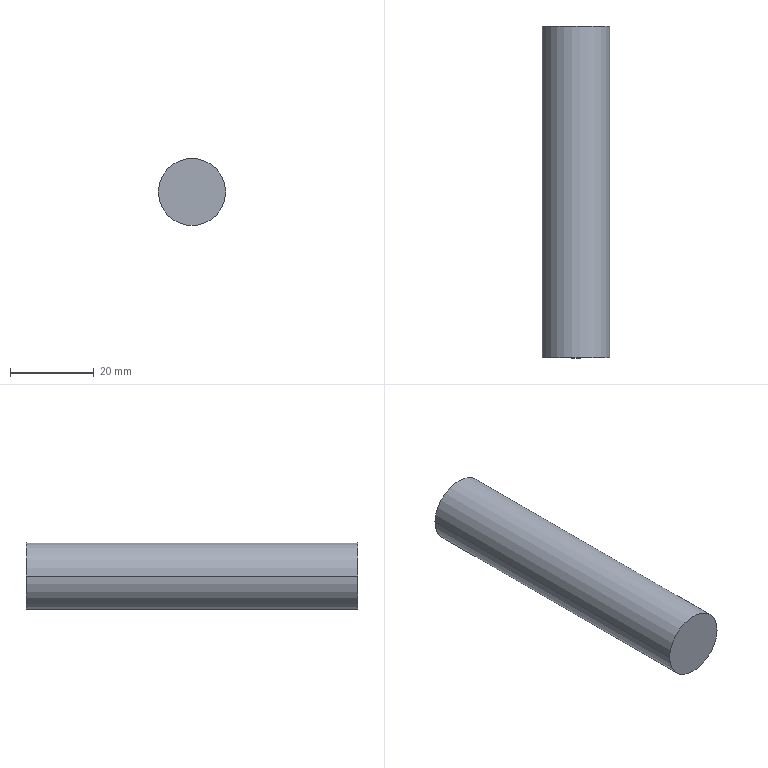Part | STEP file | copper tube 45_default_machined_ | 1 solid | 4 faces | box 16 x 79.107 x 16 mm | volume 15905 mm3 | cylinder 2 | plane 2 | commonest cylinder face diameters 16 x2
STEP:
#1=CARTESIAN_POINT('',(0.,0.,0.));
#2=DIRECTION('',(0.,0.,1.));
#3=DIRECTION('',(1.,0.,0.));
#4=AXIS2_PLACEMENT_3D('',#1,#2,#3);
#5=CARTESIAN_POINT('',(-145.405,845.5,28.193));
#6=VERTEX_POINT('',#5);
#7=CARTESIAN_POINT('',(-129.405,845.5,28.193));
#8=VERTEX_POINT('',#7);
#9=CARTESIAN_POINT('',(-137.405,845.5,28.193));
#10=DIRECTION('',(0.,1.,0.));
#11=DIRECTION('',(0.,0.,-1.));
#12=AXIS2_PLACEMENT_3D('',#9,#10,#11);
#13=CIRCLE('',#12,8.);
#14=CARTESIAN_POINT('',(-137.405,669.607,28.193));
#15=DIRECTION('',(0.,1.,0.));
#16=DIRECTION('',(-1.,0.,0.));
#17=AXIS2_PLACEMENT_3D('',#14,#15,#16);
#18=CYLINDRICAL_SURFACE('',#17,8.);
#19=CARTESIAN_POINT('',(-1.571,175.893));
#20=DIRECTION('',(1.,0.));
#21=VECTOR('',#20,1.);
#22=LINE('',#19,#21);
#23=(GEOMETRIC_REPRESENTATION_CONTEXT(2)PARAMETRIC_REPRESENTATION_CONTEXT()REPRESENTATION_CONTEXT('',''));
#24=DEFINITIONAL_REPRESENTATION('',(#22),#23);
#25=PCURVE('',#18,#24);
#26=CARTESIAN_POINT('',(0.,845.5,0.));
#27=DIRECTION('',(0.,-1.,0.));
#28=DIRECTION('',(0.,0.,-1.));
#29=AXIS2_PLACEMENT_3D('',#26,#27,#28);
#30=PLANE('',#29);
#31=CARTESIAN_POINT('',(-20.193,-137.405));
#32=CARTESIAN_POINT('',(-20.193,-151.261));
#33=CARTESIAN_POINT('',(-32.193,-144.333));
#34=CARTESIAN_POINT('',(-44.193,-137.405));
#35=CARTESIAN_POINT('',(-32.193,-130.477));
#36=CARTESIAN_POINT('',(-20.193,-123.549));
#37=CARTESIAN_POINT('',(-20.193,-137.405));
#38=(BOUNDED_CURVE()B_SPLINE_CURVE(2,(#31,#32,#33,#34,#35,#36,#37),.UNSPECIFIED.,.T.,.F.)B_SPLINE_CURVE_WITH_KNOTS((1,2,2,2,2,1),(-2.094,0.,2.094,4.189,6.283,8.378),.UNSPECIFIED.)CURVE()GEOMETRIC_REPRESENTATION_ITEM()RATIONAL_B_SPLINE_CURVE((1.,0.5,1.,0.5,1.,0.5,1.))REPRESENTATION_ITEM(''));
#39=(GEOMETRIC_REPRESENTATION_CONTEXT(2)PARAMETRIC_REPRESENTATION_CONTEXT()REPRESENTATION_CONTEXT('',''));
#40=DEFINITIONAL_REPRESENTATION('',(#38),#39);
#41=PCURVE('',#30,#40);
#42=SURFACE_CURVE('',#13,(#25,#41),.PCURVE_S1.);
#43=EDGE_CURVE('',#6,#8,#42,.T.);
#44=ORIENTED_EDGE('',*,*,#43,.T.);
#45=CARTESIAN_POINT('',(-129.405,924.607,28.193));
#46=VERTEX_POINT('',#45);
#47=CARTESIAN_POINT('',(-129.405,669.607,28.193));
#48=DIRECTION('',(0.,1.,0.));
#49=VECTOR('',#48,1.);
#50=LINE('',#47,#49);
#51=CARTESIAN_POINT('',(3.142,0.));
#52=DIRECTION('',(0.,1.));
#53=VECTOR('',#52,1.);
#54=LINE('',#51,#53);
#55=(GEOMETRIC_REPRESENTATION_CONTEXT(2)PARAMETRIC_REPRESENTATION_CONTEXT()REPRESENTATION_CONTEXT('',''));
#56=DEFINITIONAL_REPRESENTATION('',(#54),#55);
#57=PCURVE('',#18,#56);
#58=CARTESIAN_POINT('',(-137.405,669.607,28.193));
#59=DIRECTION('',(0.,1.,0.));
#60=DIRECTION('',(-1.,0.,0.));
#61=AXIS2_PLACEMENT_3D('',#58,#59,#60);
#62=CYLINDRICAL_SURFACE('',#61,8.);
#63=CARTESIAN_POINT('',(3.142,0.));
#64=DIRECTION('',(0.,1.));
#65=VECTOR('',#64,1.);
#66=LINE('',#63,#65);
#67=(GEOMETRIC_REPRESENTATION_CONTEXT(2)PARAMETRIC_REPRESENTATION_CONTEXT()REPRESENTATION_CONTEXT('',''));
#68=DEFINITIONAL_REPRESENTATION('',(#66),#67);
#69=PCURVE('',#62,#68);
#70=SURFACE_CURVE('',#50,(#57,#69),.PCURVE_S1.);
#71=EDGE_CURVE('',#8,#46,#70,.T.);
#72=ORIENTED_EDGE('',*,*,#71,.T.);
#73=CARTESIAN_POINT('',(-145.405,924.607,28.193));
#74=VERTEX_POINT('',#73);
#75=CARTESIAN_POINT('',(-137.405,924.607,28.193));
#76=DIRECTION('',(0.,1.,0.));
#77=DIRECTION('',(0.,0.,1.));
#78=AXIS2_PLACEMENT_3D('',#75,#76,#77);
#79=CIRCLE('',#78,8.);
#80=CARTESIAN_POINT('',(-4.712,255.));
#81=DIRECTION('',(1.,0.));
#82=VECTOR('',#81,1.);
#83=LINE('',#80,#82);
#84=(GEOMETRIC_REPRESENTATION_CONTEXT(2)PARAMETRIC_REPRESENTATION_CONTEXT()REPRESENTATION_CONTEXT('',''));
#85=DEFINITIONAL_REPRESENTATION('',(#83),#84);
#86=PCURVE('',#18,#85);
#87=CARTESIAN_POINT('',(-137.405,924.607,28.193));
#88=DIRECTION('',(0.,1.,0.));
#89=DIRECTION('',(0.,0.,1.));
#90=AXIS2_PLACEMENT_3D('',#87,#88,#89);
#91=PLANE('',#90);
#92=CARTESIAN_POINT('',(0.,0.));
#93=DIRECTION('',(1.,0.));
#94=AXIS2_PLACEMENT_2D('',#92,#93);
#95=CIRCLE('',#94,8.);
#96=(GEOMETRIC_REPRESENTATION_CONTEXT(2)PARAMETRIC_REPRESENTATION_CONTEXT()REPRESENTATION_CONTEXT('',''));
#97=DEFINITIONAL_REPRESENTATION('',(#95),#96);
#98=PCURVE('',#91,#97);
#99=SURFACE_CURVE('',#79,(#86,#98),.PCURVE_S1.);
#100=EDGE_CURVE('',#74,#46,#99,.T.);
#101=ORIENTED_EDGE('',*,*,#100,.F.);
#102=CARTESIAN_POINT('',(-145.405,669.607,28.193));
#103=DIRECTION('',(0.,1.,0.));
#104=VECTOR('',#103,1.);
#105=LINE('',#102,#104);
#106=CARTESIAN_POINT('',(0.,0.));
#107=DIRECTION('',(0.,1.));
#108=VECTOR('',#107,1.);
#109=LINE('',#106,#108);
#110=(GEOMETRIC_REPRESENTATION_CONTEXT(2)PARAMETRIC_REPRESENTATION_CONTEXT()REPRESENTATION_CONTEXT('',''));
#111=DEFINITIONAL_REPRESENTATION('',(#109),#110);
#112=PCURVE('',#18,#111);
#113=CARTESIAN_POINT('',(6.283,0.));
#114=DIRECTION('',(0.,1.));
#115=VECTOR('',#114,1.);
#116=LINE('',#113,#115);
#117=(GEOMETRIC_REPRESENTATION_CONTEXT(2)PARAMETRIC_REPRESENTATION_CONTEXT()REPRESENTATION_CONTEXT('',''));
#118=DEFINITIONAL_REPRESENTATION('',(#116),#117);
#119=PCURVE('',#62,#118);
#120=SURFACE_CURVE('',#105,(#112,#119),.PCURVE_S1.);
#121=EDGE_CURVE('',#6,#74,#120,.T.);
#122=ORIENTED_EDGE('',*,*,#121,.F.);
#123=EDGE_LOOP('',(#44,#72,#101,#122));
#124=FACE_BOUND('',#123,.T.);
#125=ADVANCED_FACE('',(#124),#18,.T.);
#126=ORIENTED_EDGE('',*,*,#71,.F.);
#127=CARTESIAN_POINT('',(-137.405,845.5,28.193));
#128=DIRECTION('',(0.,1.,0.));
#129=DIRECTION('',(0.,0.,-1.));
#130=AXIS2_PLACEMENT_3D('',#127,#128,#129);
#131=CIRCLE('',#130,8.);
#132=CARTESIAN_POINT('',(-1.571,175.893));
#133=DIRECTION('',(1.,0.));
#134=VECTOR('',#133,1.);
#135=LINE('',#132,#134);
#136=(GEOMETRIC_REPRESENTATION_CONTEXT(2)PARAMETRIC_REPRESENTATION_CONTEXT()REPRESENTATION_CONTEXT('',''));
#137=DEFINITIONAL_REPRESENTATION('',(#135),#136);
#138=PCURVE('',#62,#137);
#139=CARTESIAN_POINT('',(-20.193,-137.405));
#140=CARTESIAN_POINT('',(-20.193,-151.261));
#141=CARTESIAN_POINT('',(-32.193,-144.333));
#142=CARTESIAN_POINT('',(-44.193,-137.405));
#143=CARTESIAN_POINT('',(-32.193,-130.477));
#144=CARTESIAN_POINT('',(-20.193,-123.549));
#145=CARTESIAN_POINT('',(-20.193,-137.405));
#146=(BOUNDED_CURVE()B_SPLINE_CURVE(2,(#139,#140,#141,#142,#143,#144,#145),.UNSPECIFIED.,.T.,.F.)B_SPLINE_CURVE_WITH_KNOTS((1,2,2,2,2,1),(-2.094,0.,2.094,4.189,6.283,8.378),.UNSPECIFIED.)CURVE()GEOMETRIC_REPRESENTATION_ITEM()RATIONAL_B_SPLINE_CURVE((1.,0.5,1.,0.5,1.,0.5,1.))REPRESENTATION_ITEM(''));
#147=(GEOMETRIC_REPRESENTATION_CONTEXT(2)PARAMETRIC_REPRESENTATION_CONTEXT()REPRESENTATION_CONTEXT('',''));
#148=DEFINITIONAL_REPRESENTATION('',(#146),#147);
#149=PCURVE('',#30,#148);
#150=SURFACE_CURVE('',#131,(#138,#149),.PCURVE_S1.);
#151=EDGE_CURVE('',#8,#6,#150,.T.);
#152=ORIENTED_EDGE('',*,*,#151,.T.);
#153=ORIENTED_EDGE('',*,*,#121,.T.);
#154=CARTESIAN_POINT('',(-137.405,924.607,28.193));
#155=DIRECTION('',(0.,1.,0.));
#156=DIRECTION('',(0.,0.,1.));
#157=AXIS2_PLACEMENT_3D('',#154,#155,#156);
#158=CIRCLE('',#157,8.);
#159=CARTESIAN_POINT('',(1.571,255.));
#160=DIRECTION('',(1.,0.));
#161=VECTOR('',#160,1.);
#162=LINE('',#159,#161);
#163=(GEOMETRIC_REPRESENTATION_CONTEXT(2)PARAMETRIC_REPRESENTATION_CONTEXT()REPRESENTATION_CONTEXT('',''));
#164=DEFINITIONAL_REPRESENTATION('',(#162),#163);
#165=PCURVE('',#62,#164);
#166=CARTESIAN_POINT('',(0.,0.));
#167=DIRECTION('',(1.,0.));
#168=AXIS2_PLACEMENT_2D('',#166,#167);
#169=CIRCLE('',#168,8.);
#170=(GEOMETRIC_REPRESENTATION_CONTEXT(2)PARAMETRIC_REPRESENTATION_CONTEXT()REPRESENTATION_CONTEXT('',''));
#171=DEFINITIONAL_REPRESENTATION('',(#169),#170);
#172=PCURVE('',#91,#171);
#173=SURFACE_CURVE('',#158,(#165,#172),.PCURVE_S1.);
#174=EDGE_CURVE('',#46,#74,#173,.T.);
#175=ORIENTED_EDGE('',*,*,#174,.F.);
#176=EDGE_LOOP('',(#126,#152,#153,#175));
#177=FACE_BOUND('',#176,.T.);
#178=ADVANCED_FACE('',(#177),#62,.T.);
#179=ORIENTED_EDGE('',*,*,#100,.T.);
#180=ORIENTED_EDGE('',*,*,#174,.T.);
#181=EDGE_LOOP('',(#179,#180));
#182=FACE_BOUND('',#181,.T.);
#183=ADVANCED_FACE('',(#182),#91,.T.);
#184=ORIENTED_EDGE('',*,*,#43,.F.);
#185=ORIENTED_EDGE('',*,*,#151,.F.);
#186=EDGE_LOOP('',(#184,#185));
#187=FACE_BOUND('',#186,.T.);
#188=ADVANCED_FACE('',(#187),#30,.T.);
#189=CLOSED_SHELL('',(#125,#178,#183,#188));
#190=MANIFOLD_SOLID_BREP('',#189);
#191=(LENGTH_UNIT()NAMED_UNIT(*)SI_UNIT(.MILLI.,.METRE.));
#192=UNCERTAINTY_MEASURE_WITH_UNIT(LENGTH_MEASURE(0.0000001),#191,'','');
#193=(NAMED_UNIT(*)PLANE_ANGLE_UNIT()SI_UNIT($,.RADIAN.));
#194=(NAMED_UNIT(*)SI_UNIT($,.STERADIAN.)SOLID_ANGLE_UNIT());
#195=(GEOMETRIC_REPRESENTATION_CONTEXT(3)GLOBAL_UNCERTAINTY_ASSIGNED_CONTEXT((#192))GLOBAL_UNIT_ASSIGNED_CONTEXT((#191,#193,#194))REPRESENTATION_CONTEXT('',''));
#196=ADVANCED_BREP_SHAPE_REPRESENTATION('',(#4,#190),#195);